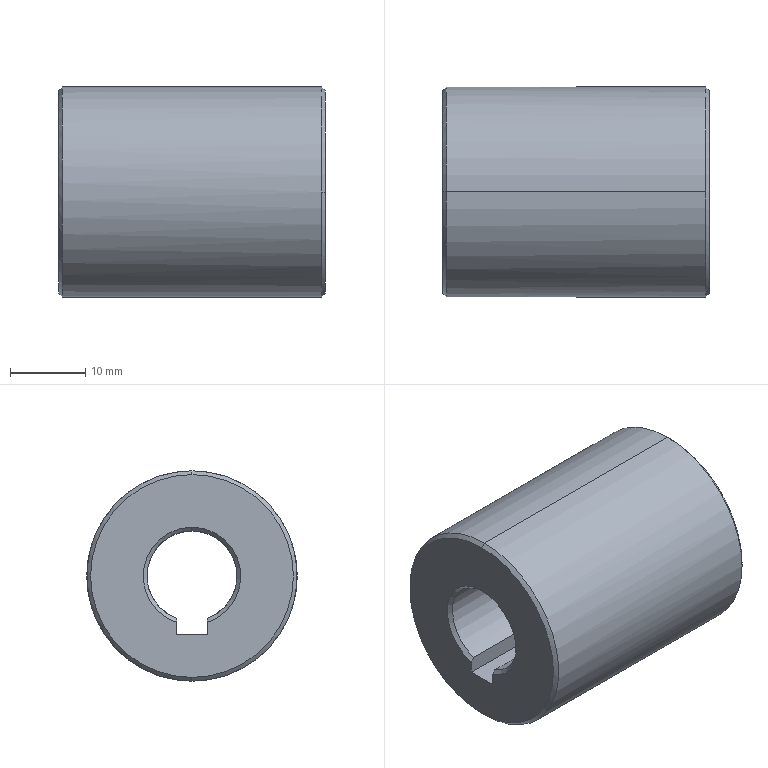Part | STEP file | PN_0037 | 1 solid | 27 faces | box 35.5 x 28 x 28 mm | volume 17402 mm3 | cone 15 | cylinder 7 | plane 5 | commonest cylinder face diameters 3.242 x4 28 x2 12 x1